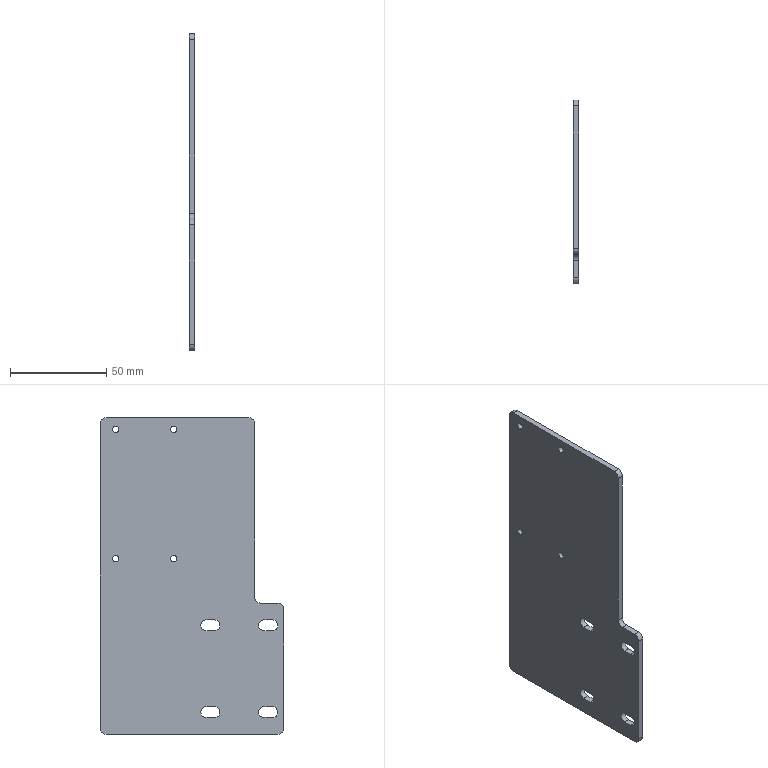Part | STEP file | cable chain hanger plate 2 | 1 solid | 38 faces | box 3 x 95 x 164 mm | volume 41712 mm3 | cylinder 22 | plane 16 | commonest cylinder face diameters 3.3 x8 5.5 x8 6 x6